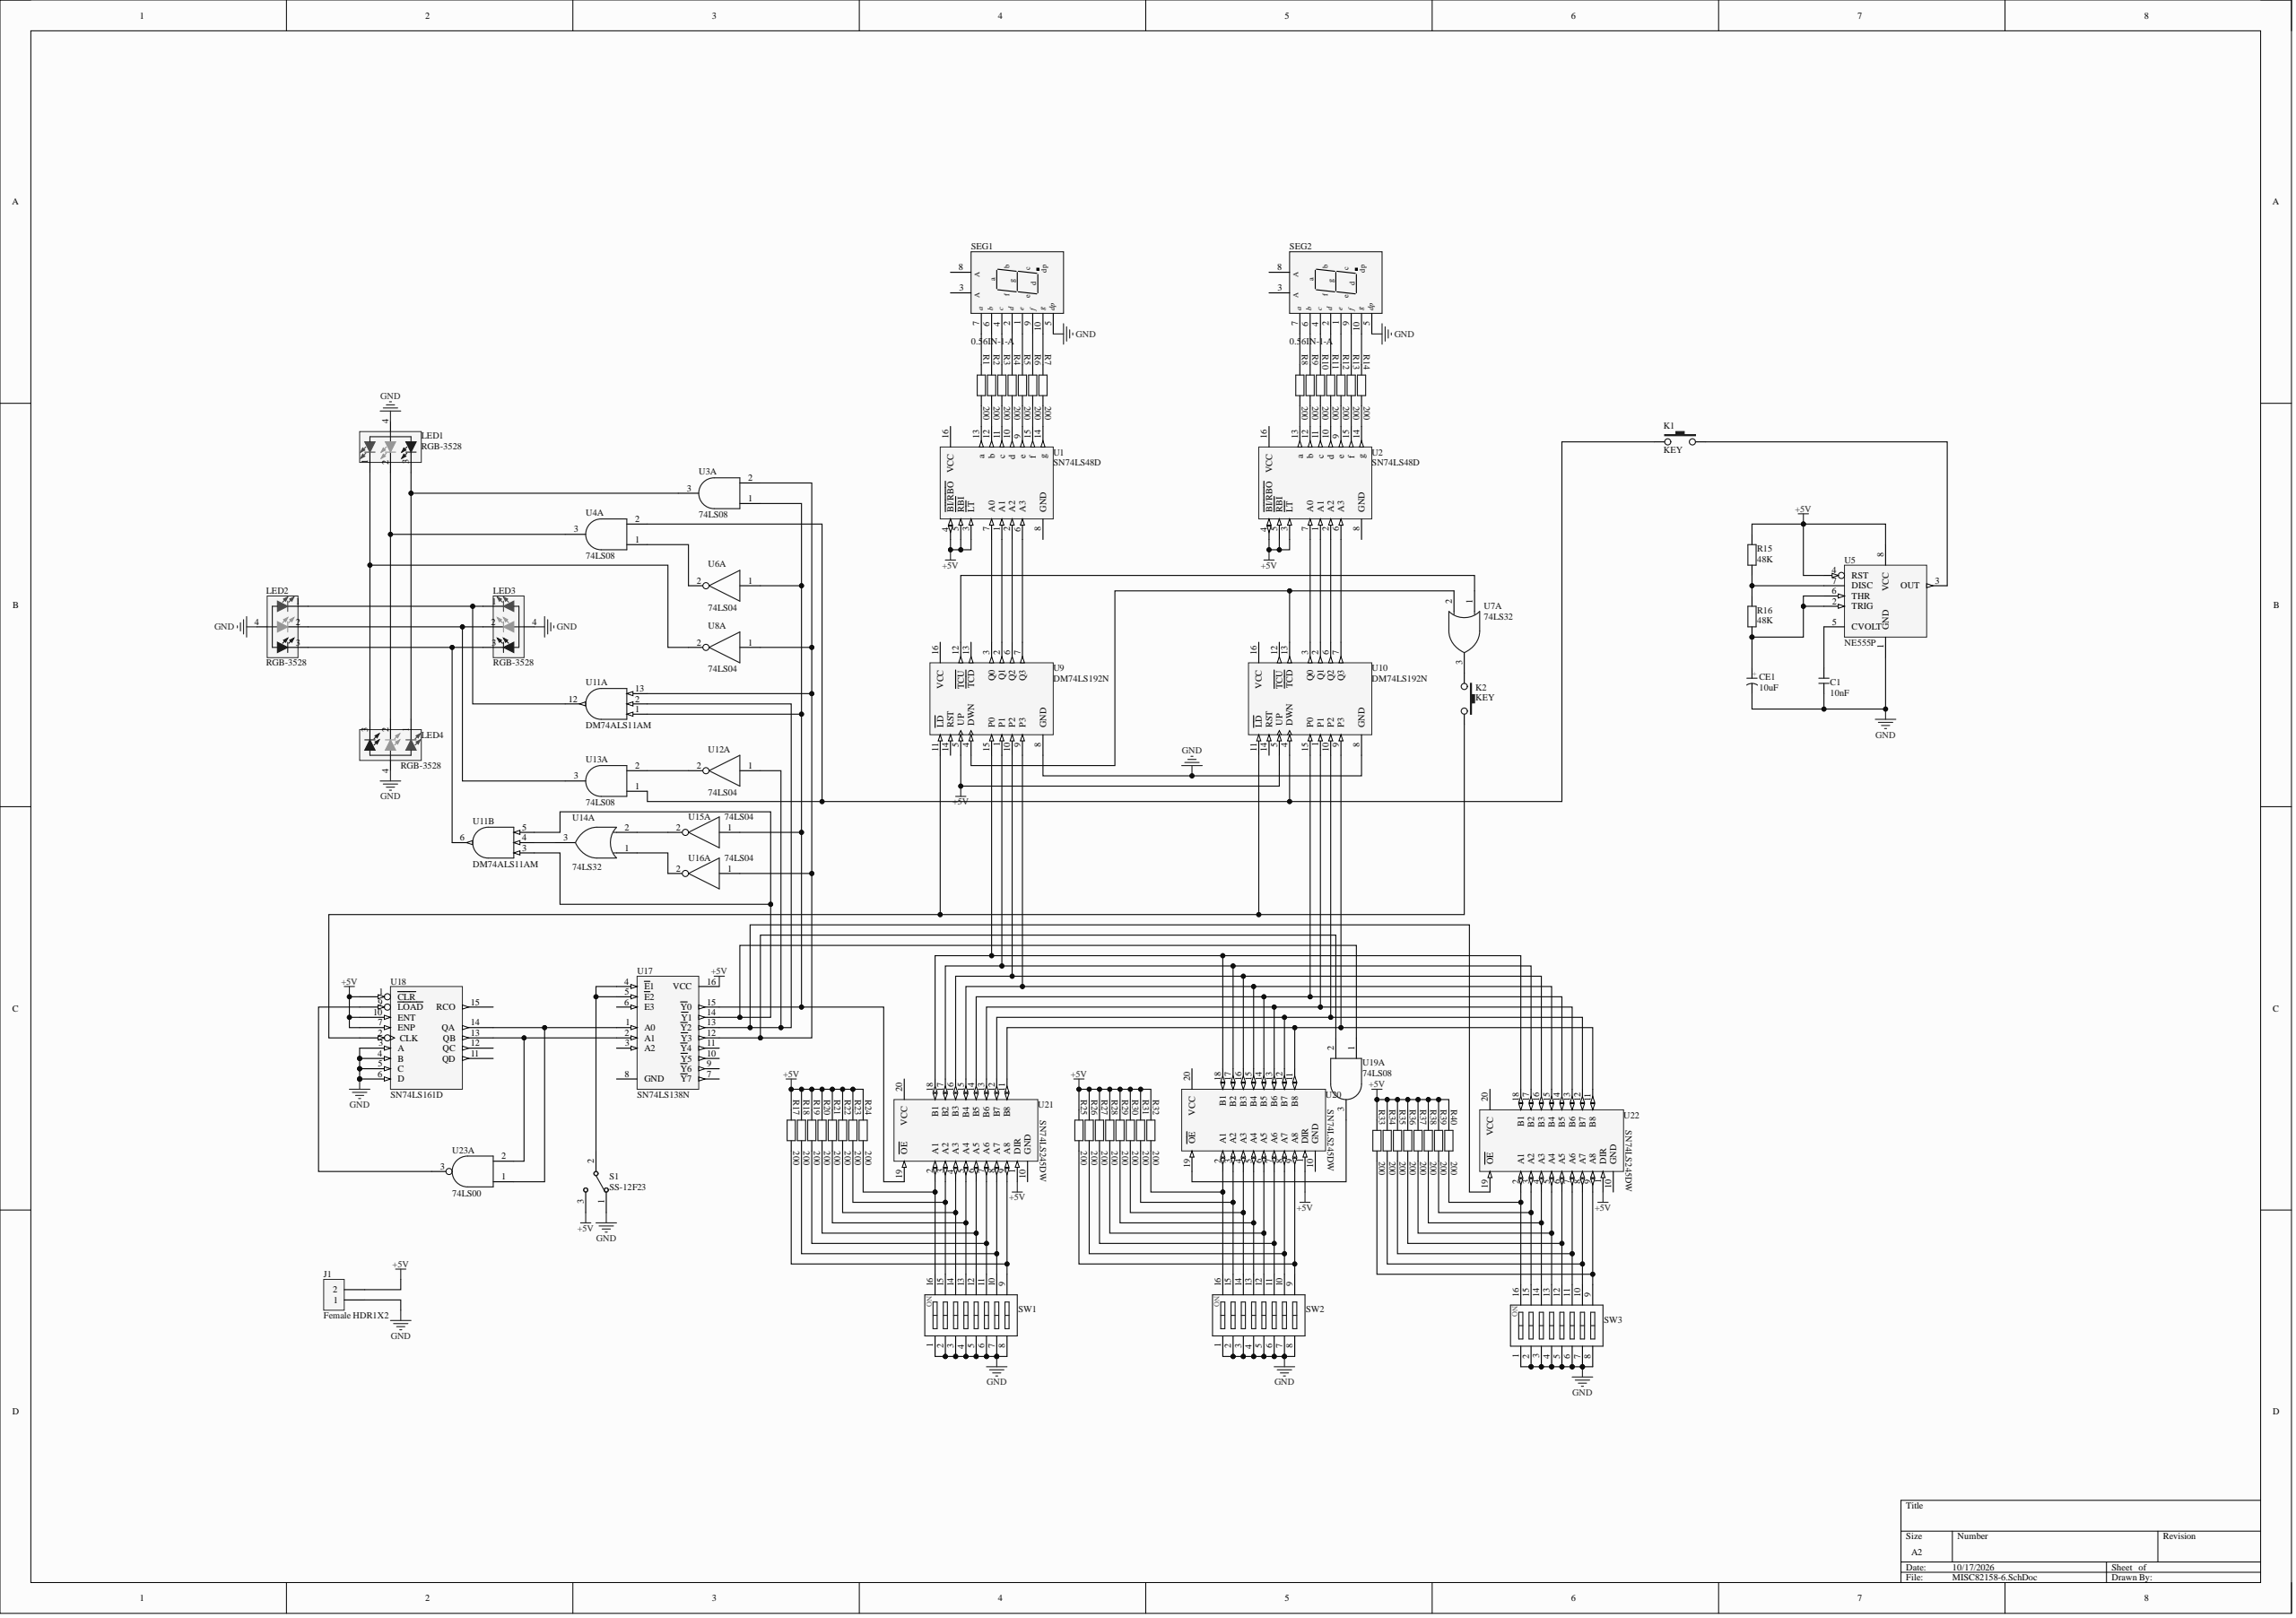Circuit board | Altium Designer | 78 parts | 100 nets
Bill of materials:
Comment,Description,Designator,Footprint,LibRef,Quantity
"10nF","Ceramic capacitor","C1","CC 1.8*3.6","CC","1"
"10uF","Through-hole electrolytic capacitor","CE1","CAP 1.5*4*8","CE","1"
"Female HDR1X2","","J1","Fe-HDR1X2/2.54-S","Female HDR1X2","1"
"KEY","","K1, K2","DIP-3X6X4.3","KEY","2"
"RGB-3528","3528 RGB LED","LED1, LED2, LED3, LED4","Fe-HDR1X4/2.54-S","LED-RGB 3528","4"
"200","Color-band resistor","R1, R2, R3, R4, R5, R6, R7, R8, R9, R10, R11, R12, R13, R14, R17, R18, R19, R20, R21, R22, R23, R24, R25, R26, R27, R28, R29, R30, R31, R32, R33, R34, R35, R36, R37, R38, R39, R40","RS 1/4W","R-S","38"
"48K","Color-band resistor","R15, R16","RS 1/4W","R-S","2"
"SS-12F23","1-way wave switch","S1","MSK-12C01-07","SSW-1P","1"
"0.56IN-1-A","1-digit 0.56 inch common-anode display","SEG1, SEG2","0.56IN-1P","0.56IN-1-A","2"
"SW-8P","8-way coded switch","SW1, SW2, SW3","CSW DIP-8P","SW-8P","3"
"SN74LS48D","BCD-to-Seven-Segment Decoder/Driver","U1, U2","SOP16","SN74LS48D","2"
"74LS08","Quad 2-input AND gate","U3, U4, U13, U19","DIP14","74LS08","4"
"NE555P","Precision Timer","U5","DIP8","NE555P","1"
"74LS04","Hex inverter","U6, U8, U12, U15, U16","DIP14","74LS04","5"
"74LS32","Quad 2-input OR gate","U7, U14","DIP14","74LS32","2"
"DM74LS192N","Up/Down Decade Counter with Separate Up/Down Clock","U9, U10","DIP16","DM74LS192N","2"
"DM74ALS11AM","Triple 3-Input AND Gate","U11","DIP16","DM74ALS11AM","1"
"SN74LS138N","1-of-8 Decoder/Demultiplexer","U17","DIP16","SN74LS138N","1"
"SN74LS161D","SYN 4-BIT CNT","U18","DIP16","SN74LS161A","1"
"SN74LS245DW","Octal Bus Transceiver","U20, U21, U22","SOP20","SN74LS245DW","3"
"74LS00","Quad 2-input NAND gate","U23","DIP14","74LS00","1"
Netlist (Protel format):
[
C1
CC 1.8*3.6
10nF



]
[
CE1
CAP 1.5*4*8
10uF



]
[
J1
Fe-HDR1X2/2.54-S
Female HDR1X2



]
[
K1
DIP-3X6X4.3
KEY



]
[
K2
DIP-3X6X4.3
KEY



]
[
LED1
Fe-HDR1X4/2.54-S
RGB-3528



]
[
LED2
Fe-HDR1X4/2.54-S
RGB-3528



]
[
LED3
Fe-HDR1X4/2.54-S
RGB-3528



]
[
LED4
Fe-HDR1X4/2.54-S
RGB-3528



]
[
R1
RS 1/4W
200



]
[
R2
RS 1/4W
200



]
[
R3
RS 1/4W
200



]
[
R4
RS 1/4W
200



]
[
R5
RS 1/4W
200



]
[
R6
RS 1/4W
200



]
[
R7
RS 1/4W
200



]
[
R8
RS 1/4W
200



]
[
R9
RS 1/4W
200



]
[
R10
RS 1/4W
200



]
[
R11
RS 1/4W
200



]
[
R12
RS 1/4W
200



]
[
R13
RS 1/4W
200



]
[
R14
RS 1/4W
200



]
[
R15
RS 1/4W
48K



]
[
R16
RS 1/4W
48K



]
[
R17
RS 1/4W
200



]
[
R18
RS 1/4W
200



]
[
R19
RS 1/4W
200



]
[
R20
RS 1/4W
200



]
[
R21
RS 1/4W
200



]
[
R22
RS 1/4W
200



]
[
R23
RS 1/4W
200



]
[
R24
RS 1/4W
200



]
[
R25
RS 1/4W
200



]
[
R26
RS 1/4W
200



]
[
R27
RS 1/4W
200



]
[
R28
RS 1/4W
200



]
[
R29
RS 1/4W
200



]
[
R30
RS 1/4W
200



]
[
R31
RS 1/4W
200



]
[
R32
RS 1/4W
200



]
[
R33
RS 1/4W
200



]
[
R34
RS 1/4W
200



]
[
R35
RS 1/4W
200



]
[
R36
RS 1/4W
200



]
[
R37
RS 1/4W
200



]
[
R38
RS 1/4W
200



]
[
R39
RS 1/4W
200



]
[
R40
RS 1/4W
200



]
[
S1
MSK-12C01-07
SS-12F23



]
[
SEG1
0.56IN-1P
0.56IN-1-A



]
[
SEG2
0.56IN-1P
0.56IN-1-A



]
[
SW1
CSW DIP-8P
SW-8P



]
[
SW2
CSW DIP-8P
SW-8P



]
[
SW3
CSW DIP-8P
SW-8P



]
[
U1
SOP16
SN74LS48D



]
[
U2
SOP16
SN74LS48D



]
[
U3
DIP14
74LS08



]
[
U4
DIP14
74LS08



]
[
U5
DIP8
NE555P



]
[
U6
DIP14
74LS04



]
[
U7
DIP14
74LS32



]
[
U8
DIP14
74LS04



]
[
U9
DIP16
DM74LS192N



]
[
U10
DIP16
DM74LS192N



]
[
U11
DIP16
DM74ALS11AM



]
[
U12
DIP14
74LS04



]
[
U13
DIP14
74LS08



]
[
U14
DIP14
74LS32



]
[
U15
DIP14
74LS04



]
[
U16
DIP14
74LS04



]
[
U17
DIP16
SN74LS138N



]
[
U18
DIP16
SN74LS161D



]
[
U19
DIP14
74LS08



]
[
U20
SOP20
SN74LS245DW



]
[
U21
SOP20
SN74LS245DW



]
[
U22
SOP20
SN74LS245DW



]
[
U23
DIP14
74LS00



]
(
VCC
U11-14
U18-16
)
(
NetU19_3
U19-3
U20-19
)
(
NetU18_9
U18-9
U23-3
)
(
NetU17_2
U17-2
U18-13
U23-2
)
(
NetU17_1
U17-1
U18-14
U23-1
)
(
NetU14_2
U14-2
U15-2
)
(
NetU14_1
U14-1
U16-2
)
(
NetU12_2
U12-2
U13-2
)
(
NetU11_4
U11-4
U14-3
)
(
NetU11_3
U11-3
U11-5
U17-14
U19-1
)
(
NetU11_2
U11-2
U12-1
U17-13
U22-19
)
(
NetU10_15
U10-15
U20-14
U21-14
U22-14
)
(
NetU10_10
U10-10
U20-12
U21-12
U22-12
)
(
NetU10_9
U10-9
U20-11
U21-11
U22-11
)
(
NetU10_1
U10-1
U20-13
U21-13
U22-13
)
(
NetU9_15
U9-15
U20-18
U21-18
U22-18
)
(
NetU9_10
U9-10
U20-16
U21-16
U22-16
)
(
NetU9_9
U9-9
U20-15
U21-15
U22-15
)
(
NetU9_1
U9-1
U20-17
U21-17
U22-17
)
(
NetU7_2
U7-2
U9-4
U10-13
)
(
NetU7_1
U7-1
U9-12
)
(
NetU4_1
U4-1
U6-2
)
(
NetU3_2
U3-2
U8-1
U11-13
U16-1
U17-12
U19-2
)
(
NetU3_1
U3-1
U6-1
U11-1
U15-1
U17-15
U21-19
)
(
NetU2_7
U2-7
U10-3
)
(
NetU2_6
U2-6
U10-7
)
(
NetU2_2
U2-2
U10-6
)
(
NetU2_1
U2-1
U10-2
)
(
NetU1_7
U1-7
U9-3
)
(
NetU1_6
U1-6
U9-7
)
(
NetU1_2
U1-2
U9-6
)
(
NetU1_1
U1-1
U9-2
)
(
NetS1_2
S1-2
U17-4
U17-5
)
(
NetR40_1
R40-1
SW3-16
U22-2
)
(
NetR39_1
R39-1
SW3-15
U22-3
)
(
NetR38_1
R38-1
SW3-14
U22-4
)
(
NetR37_1
R37-1
SW3-13
U22-5
)
(
NetR36_1
R36-1
SW3-12
U22-6
)
(
NetR35_1
R35-1
SW3-11
U22-7
)
(
NetR34_1
R34-1
SW3-10
U22-8
)
(
NetR33_1
R33-1
SW3-9
U22-9
)
(
NetR32_1
R32-1
SW2-16
U20-2
)
(
NetR31_1
R31-1
SW2-15
U20-3
)
(
NetR30_1
R30-1
SW2-14
U20-4
)
(
NetR29_1
R29-1
SW2-13
U20-5
)
(
NetR28_1
R28-1
SW2-12
U20-6
)
(
NetR27_1
R27-1
SW2-11
U20-7
)
(
NetR26_1
R26-1
SW2-10
U20-8
)
(
NetR25_1
R25-1
SW2-9
U20-9
)
(
NetR24_1
R24-1
SW1-16
U21-2
)
(
NetR23_1
R23-1
SW1-15
U21-3
)
(
NetR22_1
R22-1
SW1-14
U21-4
)
(
NetR21_1
R21-1
SW1-13
U21-5
)
(
NetR20_1
R20-1
SW1-12
U21-6
)
(
NetR19_1
R19-1
SW1-11
U21-7
)
(
NetR18_1
R18-1
SW1-10
U21-8
)
(
NetR17_1
R17-1
SW1-9
U21-9
)
(
NetR15_2
R15-2
R16-1
U5-7
)
(
NetR14_2
R14-2
SEG2-10
)
(
NetR14_1
R14-1
U2-14
)
(
NetR13_2
R13-2
SEG2-9
)
(
NetR13_1
R13-1
U2-15
)
(
NetR12_2
R12-2
SEG2-1
)
(
NetR12_1
R12-1
U2-9
)
(
NetR11_2
R11-2
SEG2-2
)
(
NetR11_1
R11-1
U2-10
)
(
NetR10_2
R10-2
SEG2-4
)
(
NetR10_1
R10-1
U2-11
)
(
NetR9_2
R9-2
SEG2-6
)
(
NetR9_1
R9-1
U2-12
)
(
NetR8_2
R8-2
SEG2-7
)
(
NetR8_1
R8-1
U2-13
)
(
NetR7_2
R7-2
SEG1-10
)
(
NetR7_1
R7-1
U1-14
)
(
NetR6_2
R6-2
SEG1-9
)
(
NetR6_1
R6-1
U1-15
)
(
NetR5_2
R5-2
SEG1-1
)
(
NetR5_1
R5-1
U1-9
)
(
NetR4_2
R4-2
SEG1-2
)
(
NetR4_1
R4-1
U1-10
)
(
NetR3_2
R3-2
SEG1-4
)
(
NetR3_1
R3-1
U1-11
)
(
NetR2_2
R2-2
SEG1-6
)
(
NetR2_1
R2-1
U1-12
)
(
NetR1_2
R1-2
SEG1-7
)
(
NetR1_1
R1-1
U1-13
)
(
NetLED2_3
LED2-3
LED3-3
U11-6
)
(
NetLED2_2
LED2-2
LED3-2
U13-3
)
(
NetLED2_1
LED2-1
LED3-1
U11-12
)
(
NetLED1_3
LED1-3
LED4-1
U3-3
)
(
NetLED1_2
LED1-2
LED4-2
U4-3
)
(
NetLED1_1
LED1-1
LED4-3
U8-2
)
(
NetK2_3
K2-3
U9-11
U10-11
U18-2
)
(
NetK2_1
K2-1
U7-3
)
(
NetK1_3
K1-3
U5-3
)
(
NetK1_1
K1-1
U4-2
U10-4
U13-1
)
(
NetCE1_1
CE1-1
R16-2
U5-2
U5-6
)
(
NetC1_2
C1-2
U5-5
)
(
GND
C1-1
CE1-2
J1-1
LED1-4
LED2-4
LED3-4
LED4-4
S1-1
SEG1-5
SEG2-5
SW1-1
SW1-2
SW1-3
SW1-4
SW1-5
SW1-6
SW1-7
SW1-8
SW2-1
SW2-2
SW2-3
SW2-4
SW2-5
SW2-6
SW2-7
SW2-8
SW3-1
SW3-2
SW3-3
SW3-4
SW3-5
SW3-6
SW3-7
SW3-8
U5-1
U9-8
U10-8
U11-7
U18-3
U18-4
U18-5
U18-6
U18-8
)
(
+5V
J1-2
R15-1
R17-2
R18-2
R19-2
R20-2
R21-2
R22-2
R23-2
R24-2
R25-2
R26-2
R27-2
R28-2
R29-2
R30-2
R31-2
R32-2
R33-2
R34-2
R35-2
R36-2
R37-2
R38-2
R39-2
R40-2
S1-3
U1-3
U1-4
U1-5
U2-3
U2-4
U2-5
U5-4
U5-8
U9-5
U10-5
U17-16
U18-1
U18-7
U18-10
U20-1
U21-1
U22-1
)